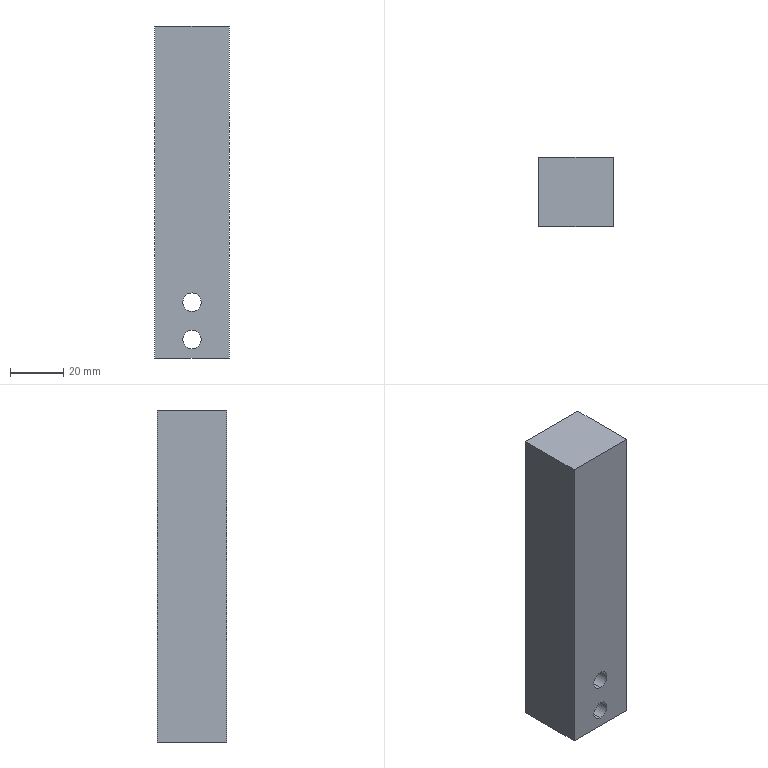Part | STEP file | xzz-Auxiliary Guide Rail | 1 solid | 16 faces | box 28 x 26 x 125 mm | volume 88103 mm3 | cylinder 8 | plane 8 | commonest cylinder face diameters 7 x4 12 x4
STEP:
#1=CARTESIAN_POINT('',(-11.37,-14.188,10.5));
#2=VERTEX_POINT('',#1);
#3=CARTESIAN_POINT('',(-11.37,-14.188,3.5));
#4=VERTEX_POINT('',#3);
#5=CARTESIAN_POINT('',(-11.37,-14.188,7.));
#6=DIRECTION('',(0.,-1.,0.));
#7=DIRECTION('',(0.,0.,1.));
#8=AXIS2_PLACEMENT_3D('',#5,#6,#7);
#9=CIRCLE('',#8,3.5);
#10=EDGE_CURVE('',#2,#4,#9,.T.);
#11=ORIENTED_EDGE('',*,*,#10,.T.);
#12=CARTESIAN_POINT('',(-11.37,5.812,3.5));
#13=VERTEX_POINT('',#12);
#14=CARTESIAN_POINT('',(-11.37,-38.188,3.5));
#15=DIRECTION('',(0.,1.,0.));
#16=VECTOR('',#15,1000.);
#17=LINE('',#14,#16);
#18=EDGE_CURVE('',#4,#13,#17,.T.);
#19=ORIENTED_EDGE('',*,*,#18,.T.);
#20=CARTESIAN_POINT('',(-11.37,5.812,10.5));
#21=VERTEX_POINT('',#20);
#22=CARTESIAN_POINT('',(-11.37,5.812,7.));
#23=DIRECTION('',(0.,-1.,0.));
#24=DIRECTION('',(0.,0.,1.));
#25=AXIS2_PLACEMENT_3D('',#22,#23,#24);
#26=CIRCLE('',#25,3.5);
#27=EDGE_CURVE('',#21,#13,#26,.T.);
#28=ORIENTED_EDGE('',*,*,#27,.F.);
#29=CARTESIAN_POINT('',(-11.37,-38.188,10.5));
#30=DIRECTION('',(0.,1.,0.));
#31=VECTOR('',#30,1000.);
#32=LINE('',#29,#31);
#33=EDGE_CURVE('',#2,#21,#32,.T.);
#34=ORIENTED_EDGE('',*,*,#33,.F.);
#35=EDGE_LOOP('',(#11,#19,#28,#34));
#36=FACE_OUTER_BOUND('',#35,.T.);
#37=CARTESIAN_POINT('',(-11.37,-38.188,7.));
#38=DIRECTION('',(0.,1.,0.));
#39=DIRECTION('',(0.,0.,1.));
#40=AXIS2_PLACEMENT_3D('',#37,#38,#39);
#41=CYLINDRICAL_SURFACE('',#40,3.5);
#42=ADVANCED_FACE('',(#36),#41,.F.);
#43=CARTESIAN_POINT('',(-11.37,-14.188,24.5));
#44=VERTEX_POINT('',#43);
#45=CARTESIAN_POINT('',(-11.37,-14.188,17.5));
#46=VERTEX_POINT('',#45);
#47=CARTESIAN_POINT('',(-11.37,-14.188,21.));
#48=DIRECTION('',(0.,-1.,0.));
#49=DIRECTION('',(0.,0.,1.));
#50=AXIS2_PLACEMENT_3D('',#47,#48,#49);
#51=CIRCLE('',#50,3.5);
#52=EDGE_CURVE('',#44,#46,#51,.T.);
#53=ORIENTED_EDGE('',*,*,#52,.T.);
#54=CARTESIAN_POINT('',(-11.37,5.812,17.5));
#55=VERTEX_POINT('',#54);
#56=CARTESIAN_POINT('',(-11.37,-38.188,17.5));
#57=DIRECTION('',(0.,1.,0.));
#58=VECTOR('',#57,1000.);
#59=LINE('',#56,#58);
#60=EDGE_CURVE('',#46,#55,#59,.T.);
#61=ORIENTED_EDGE('',*,*,#60,.T.);
#62=CARTESIAN_POINT('',(-11.37,5.812,24.5));
#63=VERTEX_POINT('',#62);
#64=CARTESIAN_POINT('',(-11.37,5.812,21.));
#65=DIRECTION('',(0.,-1.,0.));
#66=DIRECTION('',(0.,0.,1.));
#67=AXIS2_PLACEMENT_3D('',#64,#65,#66);
#68=CIRCLE('',#67,3.5);
#69=EDGE_CURVE('',#63,#55,#68,.T.);
#70=ORIENTED_EDGE('',*,*,#69,.F.);
#71=CARTESIAN_POINT('',(-11.37,-38.188,24.5));
#72=DIRECTION('',(0.,1.,0.));
#73=VECTOR('',#72,1000.);
#74=LINE('',#71,#73);
#75=EDGE_CURVE('',#44,#63,#74,.T.);
#76=ORIENTED_EDGE('',*,*,#75,.F.);
#77=EDGE_LOOP('',(#53,#61,#70,#76));
#78=FACE_OUTER_BOUND('',#77,.T.);
#79=CARTESIAN_POINT('',(-11.37,-38.188,21.));
#80=DIRECTION('',(0.,1.,0.));
#81=DIRECTION('',(0.,0.,1.));
#82=AXIS2_PLACEMENT_3D('',#79,#80,#81);
#83=CYLINDRICAL_SURFACE('',#82,3.5);
#84=ADVANCED_FACE('',(#78),#83,.F.);
#85=CARTESIAN_POINT('',(-11.37,5.812,1.));
#86=VERTEX_POINT('',#85);
#87=CARTESIAN_POINT('',(-11.37,5.812,13.));
#88=VERTEX_POINT('',#87);
#89=CARTESIAN_POINT('',(-11.37,5.812,7.));
#90=DIRECTION('',(0.,1.,0.));
#91=DIRECTION('',(0.,0.,1.));
#92=AXIS2_PLACEMENT_3D('',#89,#90,#91);
#93=CIRCLE('',#92,6.);
#94=EDGE_CURVE('',#86,#88,#93,.T.);
#95=ORIENTED_EDGE('',*,*,#94,.F.);
#96=CARTESIAN_POINT('',(-11.37,11.812,1.));
#97=VERTEX_POINT('',#96);
#98=CARTESIAN_POINT('',(-11.37,5.812,1.));
#99=DIRECTION('',(0.,1.,0.));
#100=VECTOR('',#99,1000.);
#101=LINE('',#98,#100);
#102=EDGE_CURVE('',#86,#97,#101,.T.);
#103=ORIENTED_EDGE('',*,*,#102,.T.);
#104=CARTESIAN_POINT('',(-11.37,11.812,13.));
#105=VERTEX_POINT('',#104);
#106=CARTESIAN_POINT('',(-11.37,11.812,7.));
#107=DIRECTION('',(0.,1.,0.));
#108=DIRECTION('',(0.,0.,1.));
#109=AXIS2_PLACEMENT_3D('',#106,#107,#108);
#110=CIRCLE('',#109,6.);
#111=EDGE_CURVE('',#97,#105,#110,.T.);
#112=ORIENTED_EDGE('',*,*,#111,.T.);
#113=CARTESIAN_POINT('',(-11.37,5.812,13.));
#114=DIRECTION('',(0.,1.,0.));
#115=VECTOR('',#114,1000.);
#116=LINE('',#113,#115);
#117=EDGE_CURVE('',#88,#105,#116,.T.);
#118=ORIENTED_EDGE('',*,*,#117,.F.);
#119=EDGE_LOOP('',(#95,#103,#112,#118));
#120=FACE_OUTER_BOUND('',#119,.T.);
#121=CARTESIAN_POINT('',(-11.37,5.812,7.));
#122=DIRECTION('',(0.,1.,0.));
#123=DIRECTION('',(0.,0.,1.));
#124=AXIS2_PLACEMENT_3D('',#121,#122,#123);
#125=CYLINDRICAL_SURFACE('',#124,6.);
#126=ADVANCED_FACE('',(#120),#125,.F.);
#127=CARTESIAN_POINT('',(-11.37,5.812,15.));
#128=VERTEX_POINT('',#127);
#129=CARTESIAN_POINT('',(-11.37,5.812,27.));
#130=VERTEX_POINT('',#129);
#131=CARTESIAN_POINT('',(-11.37,5.812,21.));
#132=DIRECTION('',(0.,1.,0.));
#133=DIRECTION('',(0.,0.,1.));
#134=AXIS2_PLACEMENT_3D('',#131,#132,#133);
#135=CIRCLE('',#134,6.);
#136=EDGE_CURVE('',#128,#130,#135,.T.);
#137=ORIENTED_EDGE('',*,*,#136,.F.);
#138=CARTESIAN_POINT('',(-11.37,11.812,15.));
#139=VERTEX_POINT('',#138);
#140=CARTESIAN_POINT('',(-11.37,5.812,15.));
#141=DIRECTION('',(0.,1.,0.));
#142=VECTOR('',#141,1000.);
#143=LINE('',#140,#142);
#144=EDGE_CURVE('',#128,#139,#143,.T.);
#145=ORIENTED_EDGE('',*,*,#144,.T.);
#146=CARTESIAN_POINT('',(-11.37,11.812,27.));
#147=VERTEX_POINT('',#146);
#148=CARTESIAN_POINT('',(-11.37,11.812,21.));
#149=DIRECTION('',(0.,1.,0.));
#150=DIRECTION('',(0.,0.,1.));
#151=AXIS2_PLACEMENT_3D('',#148,#149,#150);
#152=CIRCLE('',#151,6.);
#153=EDGE_CURVE('',#139,#147,#152,.T.);
#154=ORIENTED_EDGE('',*,*,#153,.T.);
#155=CARTESIAN_POINT('',(-11.37,5.812,27.));
#156=DIRECTION('',(0.,1.,0.));
#157=VECTOR('',#156,1000.);
#158=LINE('',#155,#157);
#159=EDGE_CURVE('',#130,#147,#158,.T.);
#160=ORIENTED_EDGE('',*,*,#159,.F.);
#161=EDGE_LOOP('',(#137,#145,#154,#160));
#162=FACE_OUTER_BOUND('',#161,.T.);
#163=CARTESIAN_POINT('',(-11.37,5.812,21.));
#164=DIRECTION('',(0.,1.,0.));
#165=DIRECTION('',(0.,0.,1.));
#166=AXIS2_PLACEMENT_3D('',#163,#164,#165);
#167=CYLINDRICAL_SURFACE('',#166,6.);
#168=ADVANCED_FACE('',(#162),#167,.F.);
#169=CARTESIAN_POINT('',(2.63,-14.188,125.));
#170=VERTEX_POINT('',#169);
#171=CARTESIAN_POINT('',(2.63,-14.188,0.));
#172=VERTEX_POINT('',#171);
#173=CARTESIAN_POINT('',(2.63,-14.188,125.));
#174=DIRECTION('',(0.,0.,-1.));
#175=VECTOR('',#174,1000.);
#176=LINE('',#173,#175);
#177=EDGE_CURVE('',#170,#172,#176,.T.);
#178=ORIENTED_EDGE('',*,*,#177,.F.);
#179=CARTESIAN_POINT('',(-25.37,-14.188,125.));
#180=VERTEX_POINT('',#179);
#181=CARTESIAN_POINT('',(-25.37,-14.188,125.));
#182=DIRECTION('',(1.,0.,0.));
#183=VECTOR('',#182,1000.);
#184=LINE('',#181,#183);
#185=EDGE_CURVE('',#180,#170,#184,.T.);
#186=ORIENTED_EDGE('',*,*,#185,.F.);
#187=CARTESIAN_POINT('',(-25.37,-14.188,0.));
#188=VERTEX_POINT('',#187);
#189=CARTESIAN_POINT('',(-25.37,-14.188,125.));
#190=DIRECTION('',(0.,0.,1.));
#191=VECTOR('',#190,1000.);
#192=LINE('',#189,#191);
#193=EDGE_CURVE('',#188,#180,#192,.T.);
#194=ORIENTED_EDGE('',*,*,#193,.F.);
#195=CARTESIAN_POINT('',(-25.37,-14.188,0.));
#196=DIRECTION('',(-1.,0.,0.));
#197=VECTOR('',#196,1000.);
#198=LINE('',#195,#197);
#199=EDGE_CURVE('',#172,#188,#198,.T.);
#200=ORIENTED_EDGE('',*,*,#199,.F.);
#201=EDGE_LOOP('',(#178,#186,#194,#200));
#202=FACE_OUTER_BOUND('',#201,.T.);
#203=ORIENTED_EDGE('',*,*,#10,.F.);
#204=CARTESIAN_POINT('',(-11.37,-14.188,7.));
#205=DIRECTION('',(0.,-1.,0.));
#206=DIRECTION('',(0.,0.,1.));
#207=AXIS2_PLACEMENT_3D('',#204,#205,#206);
#208=CIRCLE('',#207,3.5);
#209=EDGE_CURVE('',#4,#2,#208,.T.);
#210=ORIENTED_EDGE('',*,*,#209,.F.);
#211=EDGE_LOOP('',(#203,#210));
#212=FACE_BOUND('',#211,.T.);
#213=ORIENTED_EDGE('',*,*,#52,.F.);
#214=CARTESIAN_POINT('',(-11.37,-14.188,21.));
#215=DIRECTION('',(0.,-1.,0.));
#216=DIRECTION('',(0.,0.,1.));
#217=AXIS2_PLACEMENT_3D('',#214,#215,#216);
#218=CIRCLE('',#217,3.5);
#219=EDGE_CURVE('',#46,#44,#218,.T.);
#220=ORIENTED_EDGE('',*,*,#219,.F.);
#221=EDGE_LOOP('',(#213,#220));
#222=FACE_BOUND('',#221,.T.);
#223=CARTESIAN_POINT('',(-25.37,-14.188,125.));
#224=DIRECTION('',(0.,1.,0.));
#225=DIRECTION('',(0.,0.,1.));
#226=AXIS2_PLACEMENT_3D('',#223,#224,#225);
#227=PLANE('',#226);
#228=ADVANCED_FACE('',(#202,#212,#222),#227,.F.);
#229=CARTESIAN_POINT('',(2.63,11.812,0.));
#230=VERTEX_POINT('',#229);
#231=CARTESIAN_POINT('',(-25.37,11.812,0.));
#232=VERTEX_POINT('',#231);
#233=CARTESIAN_POINT('',(0.,11.812,0.));
#234=DIRECTION('',(-1.,0.,0.));
#235=VECTOR('',#234,1000.);
#236=LINE('',#233,#235);
#237=EDGE_CURVE('',#230,#232,#236,.T.);
#238=ORIENTED_EDGE('',*,*,#237,.F.);
#239=CARTESIAN_POINT('',(2.63,0.,0.));
#240=DIRECTION('',(0.,1.,0.));
#241=VECTOR('',#240,1000.);
#242=LINE('',#239,#241);
#243=EDGE_CURVE('',#172,#230,#242,.T.);
#244=ORIENTED_EDGE('',*,*,#243,.F.);
#245=ORIENTED_EDGE('',*,*,#199,.T.);
#246=CARTESIAN_POINT('',(-25.37,0.,0.));
#247=DIRECTION('',(0.,-1.,0.));
#248=VECTOR('',#247,1000.);
#249=LINE('',#246,#248);
#250=EDGE_CURVE('',#232,#188,#249,.T.);
#251=ORIENTED_EDGE('',*,*,#250,.F.);
#252=EDGE_LOOP('',(#238,#244,#245,#251));
#253=FACE_OUTER_BOUND('',#252,.T.);
#254=CARTESIAN_POINT('',(0.,0.,0.));
#255=DIRECTION('',(0.,0.,1.));
#256=DIRECTION('',(1.,0.,0.));
#257=AXIS2_PLACEMENT_3D('',#254,#255,#256);
#258=PLANE('',#257);
#259=ADVANCED_FACE('',(#253),#258,.F.);
#260=CARTESIAN_POINT('',(2.63,11.812,125.));
#261=VERTEX_POINT('',#260);
#262=CARTESIAN_POINT('',(2.63,11.812,125.));
#263=DIRECTION('',(0.,0.,-1.));
#264=VECTOR('',#263,1000.);
#265=LINE('',#262,#264);
#266=EDGE_CURVE('',#261,#230,#265,.T.);
#267=ORIENTED_EDGE('',*,*,#266,.F.);
#268=CARTESIAN_POINT('',(2.63,11.812,125.));
#269=DIRECTION('',(0.,1.,0.));
#270=VECTOR('',#269,1000.);
#271=LINE('',#268,#270);
#272=EDGE_CURVE('',#170,#261,#271,.T.);
#273=ORIENTED_EDGE('',*,*,#272,.F.);
#274=ORIENTED_EDGE('',*,*,#177,.T.);
#275=ORIENTED_EDGE('',*,*,#243,.T.);
#276=EDGE_LOOP('',(#267,#273,#274,#275));
#277=FACE_OUTER_BOUND('',#276,.T.);
#278=CARTESIAN_POINT('',(2.63,11.812,125.));
#279=DIRECTION('',(-1.,0.,0.));
#280=DIRECTION('',(0.,-1.,0.));
#281=AXIS2_PLACEMENT_3D('',#278,#279,#280);
#282=PLANE('',#281);
#283=ADVANCED_FACE('',(#277),#282,.F.);
#284=ORIENTED_EDGE('',*,*,#272,.T.);
#285=CARTESIAN_POINT('',(-25.37,11.812,125.));
#286=VERTEX_POINT('',#285);
#287=CARTESIAN_POINT('',(0.,11.812,125.));
#288=DIRECTION('',(-1.,0.,0.));
#289=VECTOR('',#288,1000.);
#290=LINE('',#287,#289);
#291=EDGE_CURVE('',#261,#286,#290,.T.);
#292=ORIENTED_EDGE('',*,*,#291,.T.);
#293=CARTESIAN_POINT('',(-25.37,0.,125.));
#294=DIRECTION('',(0.,-1.,0.));
#295=VECTOR('',#294,1000.);
#296=LINE('',#293,#295);
#297=EDGE_CURVE('',#286,#180,#296,.T.);
#298=ORIENTED_EDGE('',*,*,#297,.T.);
#299=ORIENTED_EDGE('',*,*,#185,.T.);
#300=EDGE_LOOP('',(#284,#292,#298,#299));
#301=FACE_OUTER_BOUND('',#300,.T.);
#302=CARTESIAN_POINT('',(0.,0.,125.));
#303=DIRECTION('',(0.,0.,1.));
#304=DIRECTION('',(1.,0.,0.));
#305=AXIS2_PLACEMENT_3D('',#302,#303,#304);
#306=PLANE('',#305);
#307=ADVANCED_FACE('',(#301),#306,.T.);
#308=ORIENTED_EDGE('',*,*,#193,.T.);
#309=ORIENTED_EDGE('',*,*,#297,.F.);
#310=CARTESIAN_POINT('',(-25.37,11.812,125.));
#311=DIRECTION('',(0.,0.,1.));
#312=VECTOR('',#311,1000.);
#313=LINE('',#310,#312);
#314=EDGE_CURVE('',#232,#286,#313,.T.);
#315=ORIENTED_EDGE('',*,*,#314,.F.);
#316=ORIENTED_EDGE('',*,*,#250,.T.);
#317=EDGE_LOOP('',(#308,#309,#315,#316));
#318=FACE_OUTER_BOUND('',#317,.T.);
#319=CARTESIAN_POINT('',(-25.37,11.812,125.));
#320=DIRECTION('',(1.,0.,0.));
#321=DIRECTION('',(0.,1.,0.));
#322=AXIS2_PLACEMENT_3D('',#319,#320,#321);
#323=PLANE('',#322);
#324=ADVANCED_FACE('',(#318),#323,.F.);
#325=ORIENTED_EDGE('',*,*,#18,.F.);
#326=ORIENTED_EDGE('',*,*,#209,.T.);
#327=ORIENTED_EDGE('',*,*,#33,.T.);
#328=CARTESIAN_POINT('',(-11.37,5.812,7.));
#329=DIRECTION('',(0.,-1.,0.));
#330=DIRECTION('',(0.,0.,1.));
#331=AXIS2_PLACEMENT_3D('',#328,#329,#330);
#332=CIRCLE('',#331,3.5);
#333=EDGE_CURVE('',#13,#21,#332,.T.);
#334=ORIENTED_EDGE('',*,*,#333,.F.);
#335=EDGE_LOOP('',(#325,#326,#327,#334));
#336=FACE_OUTER_BOUND('',#335,.T.);
#337=CARTESIAN_POINT('',(-11.37,-38.188,7.));
#338=DIRECTION('',(0.,1.,0.));
#339=DIRECTION('',(0.,0.,1.));
#340=AXIS2_PLACEMENT_3D('',#337,#338,#339);
#341=CYLINDRICAL_SURFACE('',#340,3.5);
#342=ADVANCED_FACE('',(#336),#341,.F.);
#343=ORIENTED_EDGE('',*,*,#60,.F.);
#344=ORIENTED_EDGE('',*,*,#219,.T.);
#345=ORIENTED_EDGE('',*,*,#75,.T.);
#346=CARTESIAN_POINT('',(-11.37,5.812,21.));
#347=DIRECTION('',(0.,-1.,0.));
#348=DIRECTION('',(0.,0.,1.));
#349=AXIS2_PLACEMENT_3D('',#346,#347,#348);
#350=CIRCLE('',#349,3.5);
#351=EDGE_CURVE('',#55,#63,#350,.T.);
#352=ORIENTED_EDGE('',*,*,#351,.F.);
#353=EDGE_LOOP('',(#343,#344,#345,#352));
#354=FACE_OUTER_BOUND('',#353,.T.);
#355=CARTESIAN_POINT('',(-11.37,-38.188,21.));
#356=DIRECTION('',(0.,1.,0.));
#357=DIRECTION('',(0.,0.,1.));
#358=AXIS2_PLACEMENT_3D('',#355,#356,#357);
#359=CYLINDRICAL_SURFACE('',#358,3.5);
#360=ADVANCED_FACE('',(#354),#359,.F.);
#361=ORIENTED_EDGE('',*,*,#314,.T.);
#362=ORIENTED_EDGE('',*,*,#291,.F.);
#363=ORIENTED_EDGE('',*,*,#266,.T.);
#364=ORIENTED_EDGE('',*,*,#237,.T.);
#365=EDGE_LOOP('',(#361,#362,#363,#364));
#366=FACE_OUTER_BOUND('',#365,.T.);
#367=CARTESIAN_POINT('',(-11.37,11.812,7.));
#368=DIRECTION('',(0.,1.,0.));
#369=DIRECTION('',(0.,0.,1.));
#370=AXIS2_PLACEMENT_3D('',#367,#368,#369);
#371=CIRCLE('',#370,6.);
#372=EDGE_CURVE('',#105,#97,#371,.T.);
#373=ORIENTED_EDGE('',*,*,#372,.F.);
#374=ORIENTED_EDGE('',*,*,#111,.F.);
#375=EDGE_LOOP('',(#373,#374));
#376=FACE_BOUND('',#375,.T.);
#377=CARTESIAN_POINT('',(-11.37,11.812,21.));
#378=DIRECTION('',(0.,1.,0.));
#379=DIRECTION('',(0.,0.,1.));
#380=AXIS2_PLACEMENT_3D('',#377,#378,#379);
#381=CIRCLE('',#380,6.);
#382=EDGE_CURVE('',#147,#139,#381,.T.);
#383=ORIENTED_EDGE('',*,*,#382,.F.);
#384=ORIENTED_EDGE('',*,*,#153,.F.);
#385=EDGE_LOOP('',(#383,#384));
#386=FACE_BOUND('',#385,.T.);
#387=CARTESIAN_POINT('',(-25.37,11.812,125.));
#388=DIRECTION('',(0.,-1.,0.));
#389=DIRECTION('',(0.,0.,-1.));
#390=AXIS2_PLACEMENT_3D('',#387,#388,#389);
#391=PLANE('',#390);
#392=ADVANCED_FACE('',(#366,#376,#386),#391,.F.);
#393=ORIENTED_EDGE('',*,*,#27,.T.);
#394=ORIENTED_EDGE('',*,*,#333,.T.);
#395=EDGE_LOOP('',(#393,#394));
#396=FACE_BOUND('',#395,.T.);
#397=CARTESIAN_POINT('',(-11.37,5.812,7.));
#398=DIRECTION('',(0.,1.,0.));
#399=DIRECTION('',(0.,0.,1.));
#400=AXIS2_PLACEMENT_3D('',#397,#398,#399);
#401=CIRCLE('',#400,6.);
#402=EDGE_CURVE('',#88,#86,#401,.T.);
#403=ORIENTED_EDGE('',*,*,#402,.T.);
#404=ORIENTED_EDGE('',*,*,#94,.T.);
#405=EDGE_LOOP('',(#403,#404));
#406=FACE_OUTER_BOUND('',#405,.T.);
#407=CARTESIAN_POINT('',(-11.37,5.812,7.));
#408=DIRECTION('',(0.,1.,0.));
#409=DIRECTION('',(0.,0.,1.));
#410=AXIS2_PLACEMENT_3D('',#407,#408,#409);
#411=PLANE('',#410);
#412=ADVANCED_FACE('',(#396,#406),#411,.T.);
#413=ORIENTED_EDGE('',*,*,#69,.T.);
#414=ORIENTED_EDGE('',*,*,#351,.T.);
#415=EDGE_LOOP('',(#413,#414));
#416=FACE_BOUND('',#415,.T.);
#417=CARTESIAN_POINT('',(-11.37,5.812,21.));
#418=DIRECTION('',(0.,1.,0.));
#419=DIRECTION('',(0.,0.,1.));
#420=AXIS2_PLACEMENT_3D('',#417,#418,#419);
#421=CIRCLE('',#420,6.);
#422=EDGE_CURVE('',#130,#128,#421,.T.);
#423=ORIENTED_EDGE('',*,*,#422,.T.);
#424=ORIENTED_EDGE('',*,*,#136,.T.);
#425=EDGE_LOOP('',(#423,#424));
#426=FACE_OUTER_BOUND('',#425,.T.);
#427=CARTESIAN_POINT('',(-11.37,5.812,21.));
#428=DIRECTION('',(0.,1.,0.));
#429=DIRECTION('',(0.,0.,1.));
#430=AXIS2_PLACEMENT_3D('',#427,#428,#429);
#431=PLANE('',#430);
#432=ADVANCED_FACE('',(#416,#426),#431,.T.);
#433=ORIENTED_EDGE('',*,*,#102,.F.);
#434=ORIENTED_EDGE('',*,*,#402,.F.);
#435=ORIENTED_EDGE('',*,*,#117,.T.);
#436=ORIENTED_EDGE('',*,*,#372,.T.);
#437=EDGE_LOOP('',(#433,#434,#435,#436));
#438=FACE_OUTER_BOUND('',#437,.T.);
#439=CARTESIAN_POINT('',(-11.37,5.812,7.));
#440=DIRECTION('',(0.,1.,0.));
#441=DIRECTION('',(0.,0.,1.));
#442=AXIS2_PLACEMENT_3D('',#439,#440,#441);
#443=CYLINDRICAL_SURFACE('',#442,6.);
#444=ADVANCED_FACE('',(#438),#443,.F.);
#445=ORIENTED_EDGE('',*,*,#144,.F.);
#446=ORIENTED_EDGE('',*,*,#422,.F.);
#447=ORIENTED_EDGE('',*,*,#159,.T.);
#448=ORIENTED_EDGE('',*,*,#382,.T.);
#449=EDGE_LOOP('',(#445,#446,#447,#448));
#450=FACE_OUTER_BOUND('',#449,.T.);
#451=CARTESIAN_POINT('',(-11.37,5.812,21.));
#452=DIRECTION('',(0.,1.,0.));
#453=DIRECTION('',(0.,0.,1.));
#454=AXIS2_PLACEMENT_3D('',#451,#452,#453);
#455=CYLINDRICAL_SURFACE('',#454,6.);
#456=ADVANCED_FACE('',(#450),#455,.F.);
#457=CLOSED_SHELL('',(#42,#84,#126,#168,#228,#259,#283,#307,#324,#342,#360,#392,#412,#432,#444,#456));
#458=MANIFOLD_SOLID_BREP('',#457);
#459=CARTESIAN_POINT('',(0.,0.,0.));
#460=DIRECTION('',(0.,0.,1.));
#461=DIRECTION('',(1.,0.,0.));
#462=AXIS2_PLACEMENT_3D('',#459,#460,#461);
#463=(LENGTH_UNIT()NAMED_UNIT(*)SI_UNIT(.MILLI.,.METRE.));
#464=UNCERTAINTY_MEASURE_WITH_UNIT(LENGTH_MEASURE(0.00001),#463,'','');
#465=(NAMED_UNIT(*)PLANE_ANGLE_UNIT()SI_UNIT($,.RADIAN.));
#466=(NAMED_UNIT(*)SI_UNIT($,.STERADIAN.)SOLID_ANGLE_UNIT());
#467=(GEOMETRIC_REPRESENTATION_CONTEXT(3)GLOBAL_UNCERTAINTY_ASSIGNED_CONTEXT((#464))GLOBAL_UNIT_ASSIGNED_CONTEXT((#463,#465,#466))REPRESENTATION_CONTEXT('',''));
#468=ADVANCED_BREP_SHAPE_REPRESENTATION('',(#458,#462),#467);